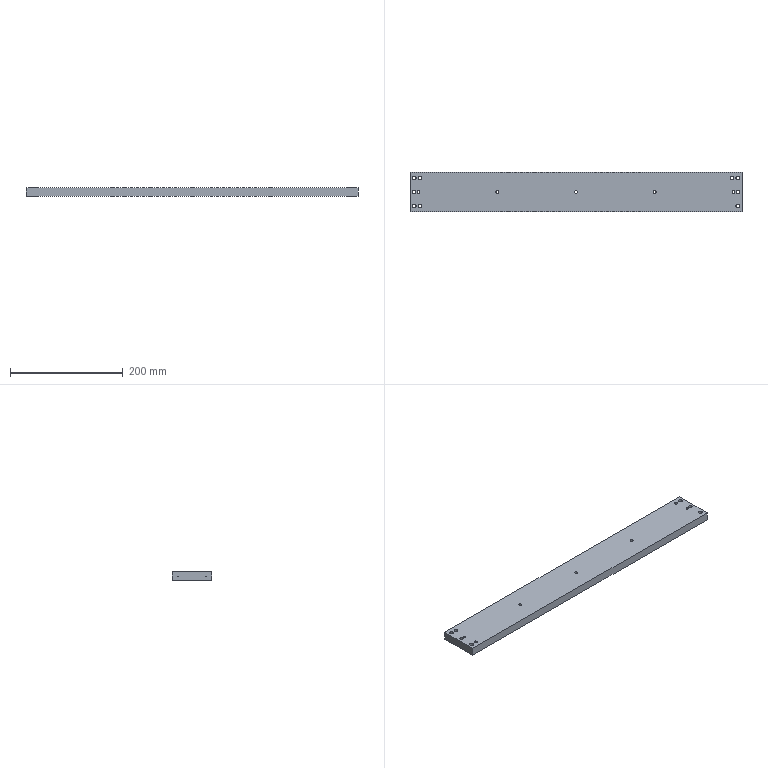CAM job | NX | 3-axis milling, drilling | part box 590 x 70 x 15 mm | stock box 590 x 70 x 15 mm
Tools:
number,name,description,diameter,corner_radius,flute_length,length,flutes
6,D6,平底铣刀-粗,6.0,0.0,25.0,75.0,2
7,D6-J,平底铣刀-精,6.0,0.0,25.0,75.0,2
2,D6倒角刀,倒角刀,6.0,0.0,3.0,25.0,2
23,M6X1.0,丝锥,5.0,0.0,35.0,50.0,2
19,D6铰刀,Drilling Tool,6.0,0.0,75.0,100.0,6
1,C6定点钻,倒角刀,6.0,0.0,3.0,3.0,2
15,ZT5.1,钻头,5.1,0.0,35.0,50.0,2
18,ZT6.6,钻头,6.6,0.0,35.0,50.0,2
17,ZT5.9,Drilling Tool,5.9,0.0,35.0,50.0,2
Operations:
program,operation,operation_type,tool,method,geometry_group,spindle_rpm,surface_speed,feed_per_tooth,feed_cut,feed_plunge,cut_length_mm,path_length_mm,cut_time_min,machine_time_min
B,CHAMFERMILL_4,PlanarMilling,D6倒角刀,METHOD,W-B,4000.0,75.398,0.0375,300.0,100.0,90.102,861.129,0.3003,0.3774
B,CHAMFERMILL_5,PlanarMilling,D6倒角刀,METHOD,W-B,4000.0,75.398,0.075,600.0,100.0,90.102,937.745,0.1502,0.2349
B,CHAMFERMILL_6,PlanarMilling,D6倒角刀,METHOD,W-B,4000.0,75.398,0.075,600.0,100.0,77.764,921.567,0.1296,0.214
B,C0.3_CLOSEDCONTOURCHAMFER6X45L_COPY_1,PlanarMilling,D6倒角刀,WALL_CHAMFER-DEPTH0-STEPG,W-B,4000.0,75.398,0.125,1000.0,100.0,1338.958,1375.158,1.339,1.343
A,SPOT-DEPTH0.8,Operation,C6定点钻,NONE,W-A,3000.0,56.0,0.01,60.0,90.0,25.2,810.073,0.42,0.4985
A,THRUHOLE-M6TAPDRILL,Operation,ZT5.1,NONE,W-A,800.0,12.566,0.0625,100.0,90.0,105.0,814.014,1.05,1.121
A,THRUHOLE-FINISH6.0PILOT_2,Operation,ZT5.9,NONE,W-A,1000.0,18.535,0.04,80.0,90.0,103.516,886.434,1.294,1.372
A,COUNTERBORE-DRILL0SEG,Operation,ZT6.6,NONE,W-A,600.0,12.441,0.1,120.0,90.0,79.931,877.884,0.6661,0.7459
A,HOLEROUGH_D6_1,CylinderMilling,D6,NONE,W-A,4000.0,75.398,0.25,2000.0,100.0,2171.652,3030.252,1.086,1.172
A,HOLEFINISH_D6_1,CylinderMilling,D6-J,FINISH-STEPDEPTH-OFF,W-A,4000.0,75.398,0.1,800.0,100.0,178.461,1039.061,0.2231,0.3091
A,CHAMFERMILL_2,PlanarMilling,D6倒角刀,METHOD,W-A,4000.0,75.398,0.05,400.0,100.0,104.819,947.328,0.262,0.3463
A,CHAMFERMILL_3,PlanarMilling,D6倒角刀,NONE,W-A,4000.0,75.398,0.1,800.0,100.0,173.57,986.733,0.217,0.2983
A,CHAMFERMILL_7,PlanarMilling,D6倒角刀,METHOD,W-A,4000.0,75.398,0.0375,300.0,100.0,99.691,865.75,0.3323,0.4089
A,C0.3_CLOSEDCONTOURCHAMFER6X45L_COPY,PlanarMilling,D6倒角刀,WALL_CHAMFER-DEPTH0-STEPG,W-A,4000.0,75.398,0.125,1000.0,100.0,1338.958,1375.158,1.339,1.343
A,REAM_2,Operation,D6铰刀,METHOD,W-A,500.0,9.425,0.0167,50.0,0.0,85.0,849.403,1.7,1.776
A,THRUHOLE-TAPM6,Operation,M6X1.0,METHOD,W-A,400.0,6.283,0.0013,1.0,90.0,97.5,799.014,97.5,97.57